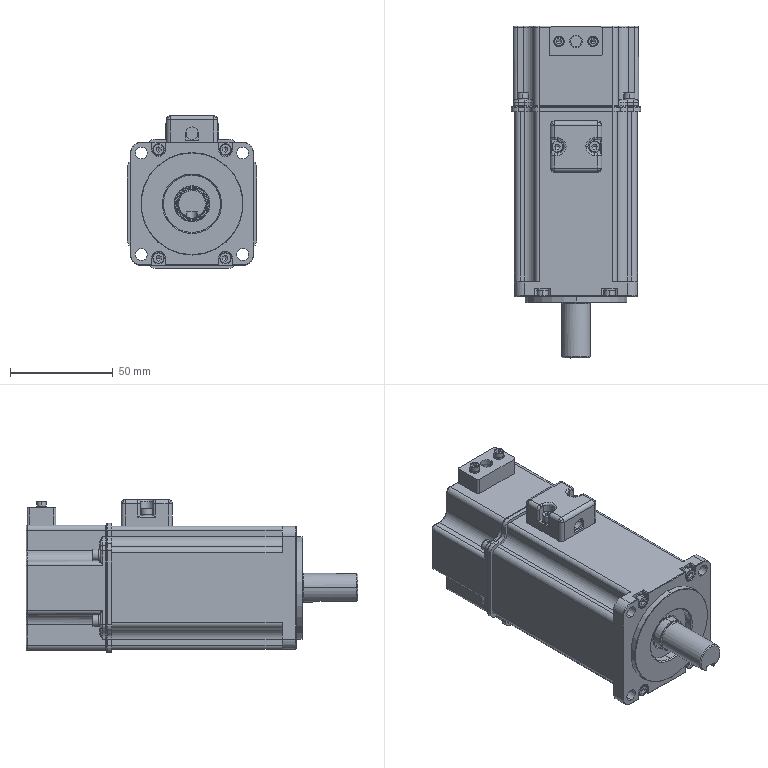Part | STEP file | 1 solid | 952 faces | box 63 x 161.8 x 74.5 mm | volume 210839 mm3 | cylinder 380 | plane 322 | spline 164 | cone 86 | commonest cylinder face diameters 1 x91 2 x31 5.5 x22 5.32 x20 4 x18 10 x13